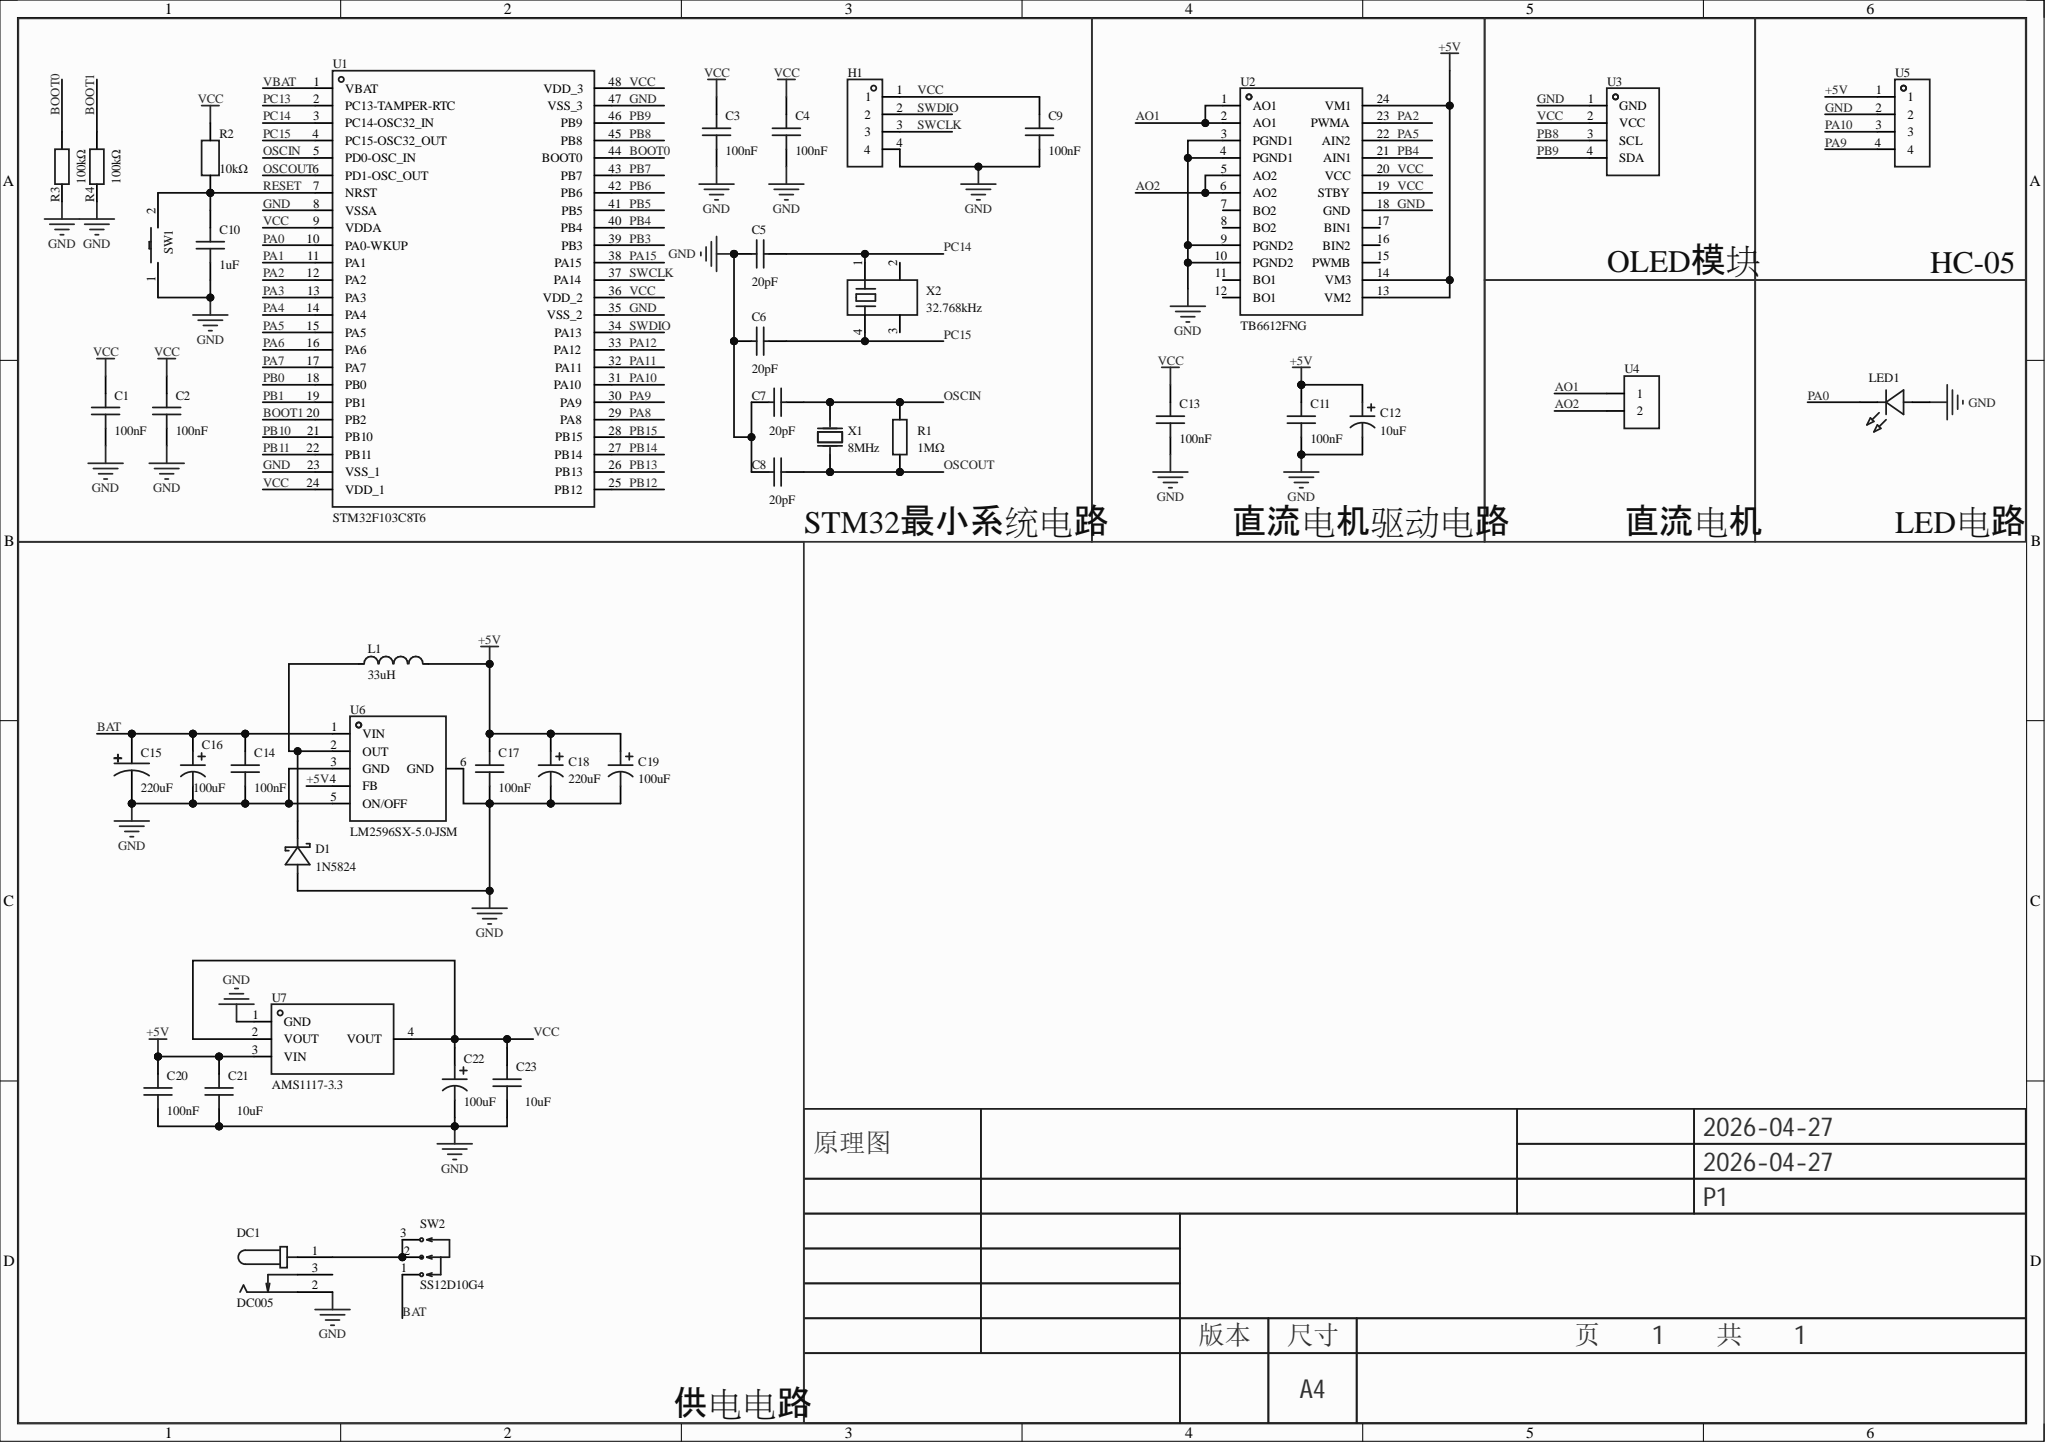Circuit board | Altium Designer | 43 parts | 25 nets
Bill of materials:
Comment,Description,Designator,Footprint,LibRef,Quantity
"100nF","容值:100nF;精度:±10%;额定电压:50V;温度系数:X7R;","C1, C2, C3, C4, C9, C11, C13, C14, C17, C20","C0603","CGA0603X7R104K500JT","10"
"20pF","容值:20pF;精度:±5%;额定电压:50V;温度系数:C0G;","C5, C6, C7, C8","C0603","CL10C200JB8NNNC","4"
"1uF","容值:1uF;精度:±10%;额定电压:50V;温度系数:X7R;","C10","C0603","CC0603KRX7R9BB105","1"
"10uF","","C12","CAP-TH_BD5.0-P2.00-D0.5-FD-A","ERG50V10M5X11","1"
"220uF","容值:220uF;精度:±20%;额定电压:50V;纹波电流:-;等效串联电阻(ESR):-;","C15","CAP-TH_BD10.0-P5.00-D1.0-FD","ECRE1013221M050P00","1"
"100uF","","C16, C19, C22","CAP-TH_BD6.3-P2.50-D0.5-FD","DXW050M107E122S1AA, 100uF16V6.3x11KM","3"
"220uF","容值:220uF;精度:±20%;额定电压:25V;纹波电流:640mA@100KHz;","C18","CAP-TH_BD6.3-P2.50-D0.5-FD_DXW025M227E112S1AA","DXW025M227E112S1AA","1"
"10uF","容值:10uF;精度:±10%;额定电压:25V;温度系数:X5R;","C21, C23","C0805","CGA0805X5R106K250MT","2"
"1N5824","","D1","DO-201AD_BD5.3-L9.0-P13.00-D1.3-RD","1N5824_C27636124","1"
"DC005","连接器类型:DC电源插座;安装方式:弯插;触点内径:2mm;触点外径:6.3mm;额定电流:500mA;额定电压:12V;工作温度:-30℃~+70℃;","DC1","DC-IN-TH_DC005","DC005","1"
"PZ254R-11-04P","插针结构:1x4P;间距:2.54mm;行距:-;圆针/方针:方针;安装方式:弯插;排数:单排;总PIN位数:4P;额定电流:3A;额定电压:250V;配合针长度:6mm;塑高:2.5mm;端接针长度:-;触头材质:黄铜;触头镀层:-;工作温度:-40℃~+105℃;颜色:黑色;","H1","HDR-TH_4P-P2.54-H-M-W10.4","PZ254R-11-04P","1"
"33uH","电感值:33uH;精度:±20%;额定电流:240mA;","L1","IND-SMD_L3.5-W3.0","YP0301-330M","1"
"BL-BUB1V4V-AT","发光颜色:红色;正向电流:-;","LED1","LED-TH_BD5.8-P2.54-FD_RED","BL-BUB1V4V-AT","1"
"1MΩ","","R1","R0603","0603WAF1004T5E","1"
"10kΩ","","R2","R0603","FRC0603F1002TS","1"
"100kΩ","","R3, R4","R0603","0603WAF1003T5E","2"
"TS-1101-C-W","电路结构:单刀单掷;按钮形状:矩形按钮;作用力:2.6N;安装方式:立贴;开关长度:6mm;开关宽度:3.6mm;开关高度:2.5mm;带支架:不带支架;触点电流:50mA;额定电压:12V;带灯:无;工作寿命:5万次;","SW1","SW-SMD_L6.0-W3.3-LS8.0_TS-1101-C-W","TS-1101-C-W","1"
"SS12D10G4","电路结构:单刀双掷;安装方式:直插;开关颜色:黑色;额定电流:2A;额定电压:125V;","SW2","SW-TH_3P-P4.80-HX-SS12D10G4","SS12D10G4","1"
"STM32F103C8T6","CPU内核:ARM-M3;CPU最大主频:72MHz;应用领域:-;","U1","LQFP-48_L7.0-W7.0-P0.50-LS9.0-BL","STM32F103C8T6","1"
"TB6612FNG","","U2","SSOP-24_L8.4-W5.8-P0.65-LS7.8-BL","TB6612FNG(O,C,8,EL","1"
"HS96L03W2C03","核心芯片:SSD1315芯片;接口类型:I2C;尺寸(inch):0.96;像素分辨率:128x64;","U3","OLED-TH_L27.8-W27.2-P2.54_C9900033791","HS96L03W2C03","1"
"2.54-1*2P母","插孔结构:1x2P;间距:2.54mm;行距:-;圆孔/方孔:方孔;安装方式:直插;排数:单排;总孔位数:2P;额定电流:3A;额定电压:-;插孔方向:顶部;塑高:-;触头材质:黄铜;触头镀层:-;工作温度:-40℃~+105℃;","U4","HDR-TH_2P-P2.54-V-F","2.54-1*2P母","1"
"2.54-1*4P母","插孔结构:1x4P;间距:2.54mm;行距:-;圆孔/方孔:方孔;安装方式:直插;排数:单排;总孔位数:4P;额定电流:3A;额定电压:-;插孔方向:顶部;塑高:-;触头材质:青铜;触头镀层:-;工作温度:-40℃~+105℃;","U5","HDR-TH_4P-P2.54-V-F","2.54-1*4P母","1"
"LM2596SX-5.0-JSM","功能类型:降压型;工作电压:5V~40V;输出电压:1.23V~37V;输出电流:3A;输出类型:固定;","U6","TO-263-5_L10.0-W8.4-P1.70-LS15.3-BR","LM2596SX-5.0-JSM","1"
"AMS1117-3.3","输出类型:固定;工作电压:15V;输出电压:3.3V;输出电流:1A;电源纹波抑制比(PSRR):72dB@(120Hz);输出极性:正极;","U7","SOT-223-3_L6.5-W3.4-P2.30-LS7.0-BR","AMS1117-3.3_C6186","1"
"8MHz","晶振类型:直插晶振;频率:8MHz;常温频差:±20ppm;负载电容:20pF;频率稳定度:±30ppm;","X1","OSC-TH_L10.0-W4.5-P5.00","X49SD8MSD2SC","1"
"32.768kHz","晶振类型:贴片晶振;频率:32.768kHz;常温频差:±20ppm;负载电容:12.5pF;","X2","MC-306_4P-L8.0-W3.2-P5.5-BL","Q13MC30610003","1"
Netlist (Protel format):
[
C1
C0603
100nF



]
[
C2
C0603
100nF



]
[
C3
C0603
100nF



]
[
C4
C0603
100nF



]
[
C5
C0603
20pF



]
[
C6
C0603
20pF



]
[
C7
C0603
20pF



]
[
C8
C0603
20pF



]
[
C9
C0603
100nF



]
[
C10
C0603
1uF



]
[
C11
C0603
100nF



]
[
C12
CAP-TH_BD5.0-P2.00-D0.5-FD-A
10uF



]
[
C13
C0603
100nF



]
[
C14
C0603
100nF



]
[
C15
CAP-TH_BD10.0-P5.00-D1.0-FD
220uF



]
[
C16
CAP-TH_BD6.3-P2.50-D0.5-FD
100uF



]
[
C17
C0603
100nF



]
[
C18
CAP-TH_BD6.3-P2.50-D0.5-FD_DXW025M227E112S1AA
220uF



]
[
C19
CAP-TH_BD6.3-P2.50-D0.5-FD
100uF



]
[
C20
C0603
100nF



]
[
C21
C0805
10uF



]
[
C22
CAP-TH_BD6.3-P2.50-D0.5-FD
100uF



]
[
C23
C0805
10uF



]
[
D1
DO-201AD_BD5.3-L9.0-P13.00-D1.3-RD
1N5824



]
[
DC1
DC-IN-TH_DC005
DC005



]
[
H1
HDR-TH_4P-P2.54-H-M-W10.4
PZ254R-11-04P



]
[
L1
IND-SMD_L3.5-W3.0
33uH



]
[
LED1
LED-TH_BD5.8-P2.54-FD_RED
BL-BUB1V4V-AT



]
[
R1
R0603
1MΩ



]
[
R2
R0603
10kΩ



]
[
R3
R0603
100kΩ



]
[
R4
R0603
100kΩ



]
[
SW1
SW-SMD_L6.0-W3.3-LS8.0_TS-1101-C-W
TS-1101-C-W



]
[
SW2
SW-TH_3P-P4.80-HX-SS12D10G4
SS12D10G4



]
[
U1
LQFP-48_L7.0-W7.0-P0.50-LS9.0-BL
STM32F103C8T6



]
[
U2
SSOP-24_L8.4-W5.8-P0.65-LS7.8-BL
TB6612FNG



]
[
U3
OLED-TH_L27.8-W27.2-P2.54_C9900033791
HS96L03W2C03



]
[
U4
HDR-TH_2P-P2.54-V-F
2.54-1*2P母



]
[
U5
HDR-TH_4P-P2.54-V-F
2.54-1*4P母



]
[
U6
TO-263-5_L10.0-W8.4-P1.70-LS15.3-BR
LM2596SX-5.0-JSM



]
[
U7
SOT-223-3_L6.5-W3.4-P2.30-LS7.0-BR
AMS1117-3.3



]
[
X1
OSC-TH_L10.0-W4.5-P5.00
8MHz



]
[
X2
MC-306_4P-L8.0-W3.2-P5.5-BL
32.768kHz



]
(
VCC
C1-2
C2-2
C3-2
C4-2
C9-2
C13-2
C22-1
C23-2
H1-1
R2-2
U1-9
U1-24
U1-36
U1-48
U2-19
U2-20
U3-2
U7-2
U7-4
)
(
SWDIO
H1-2
U1-34
)
(
SWCLK
H1-3
U1-37
)
(
RESET
C10-2
R2-1
SW1-2
U1-7
)
(
PC15
C6-1
U1-4
X2-4
)
(
PC14
C5-1
U1-3
X2-1
)
(
PB9
U1-46
U3-4
)
(
PB8
U1-45
U3-3
)
(
PB4
U1-40
U2-21
)
(
PA10
U1-31
U5-3
)
(
PA9
U1-30
U5-4
)
(
PA5
U1-15
U2-22
)
(
PA2
U1-12
U2-23
)
(
PA0
LED1-2
U1-10
)
(
OSCOUT
C8-1
R1-1
U1-6
X1-2
)
(
OSCIN
C7-1
R1-2
U1-5
X1-1
)
(
NetDC1_1
DC1-1
SW2-2
SW2-3
)
(
NetD1_1
D1-1
L1-1
U6-2
)
(
GND
C1-1
C2-1
C3-1
C4-1
C5-2
C6-2
C7-2
C8-2
C9-1
C10-1
C11-1
C12-2
C13-1
C14-1
C15-2
C16-2
C17-1
C18-2
C19-2
C20-1
C21-1
C22-2
C23-1
D1-2
DC1-2
H1-4
LED1-1
R3-1
R4-1
SW1-1
U1-8
U1-23
U1-35
U1-47
U2-3
U2-4
U2-9
U2-10
U2-18
U3-1
U5-2
U6-3
U6-5
U6-6
U7-1
)
(
BOOT1
R4-2
U1-20
)
(
BOOT0
R3-2
U1-44
)
(
BAT
C14-2
C15-1
C16-1
SW2-1
U6-1
)
(
AO2
U2-5
U2-6
U4-2
)
(
AO1
U2-1
U2-2
U4-1
)
(
+5V
C11-2
C12-1
C17-2
C18-1
C19-1
C20-2
C21-2
L1-2
U2-13
U2-14
U2-24
U5-1
U6-4
U7-3
)